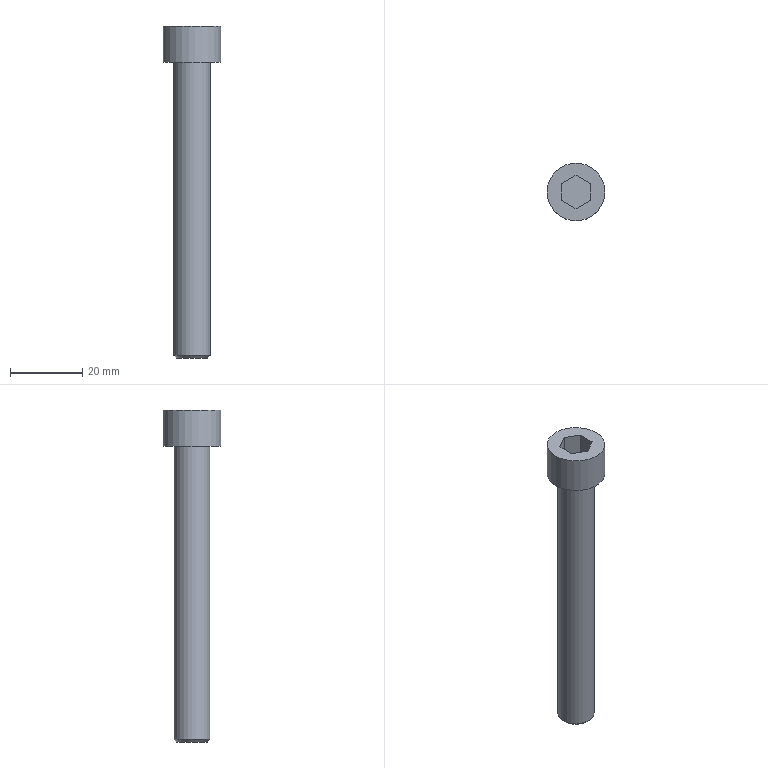Part | STEP file | gslz 2016.10.28-6_id690_x_t | 1 solid | 13 faces | box 16 x 16 x 92 mm | volume 8110 mm3 | plane 10 | cylinder 2 | cone 1 | commonest cylinder face diameters 10 x1 16 x1
STEP:
#1=CARTESIAN_POINT('',(179.7,197.309,72.));
#2=VERTEX_POINT('',#1);
#3=CARTESIAN_POINT('',(179.7,192.691,72.));
#4=VERTEX_POINT('',#3);
#5=CARTESIAN_POINT('',(179.7,197.309,72.));
#6=DIRECTION('',(0.,-1.,0.));
#7=VECTOR('',#6,1.);
#8=LINE('',#5,#7);
#9=EDGE_CURVE('',#2,#4,#8,.T.);
#10=ORIENTED_EDGE('',*,*,#9,.T.);
#11=CARTESIAN_POINT('',(175.7,190.381,72.));
#12=VERTEX_POINT('',#11);
#13=CARTESIAN_POINT('',(179.7,192.691,72.));
#14=DIRECTION('',(-0.866,-0.5,0.));
#15=VECTOR('',#14,1.);
#16=LINE('',#13,#15);
#17=EDGE_CURVE('',#4,#12,#16,.T.);
#18=ORIENTED_EDGE('',*,*,#17,.T.);
#19=CARTESIAN_POINT('',(171.7,192.691,72.));
#20=VERTEX_POINT('',#19);
#21=CARTESIAN_POINT('',(175.7,190.381,72.));
#22=DIRECTION('',(-0.866,0.5,0.));
#23=VECTOR('',#22,1.);
#24=LINE('',#21,#23);
#25=EDGE_CURVE('',#12,#20,#24,.T.);
#26=ORIENTED_EDGE('',*,*,#25,.T.);
#27=CARTESIAN_POINT('',(171.7,197.309,72.));
#28=VERTEX_POINT('',#27);
#29=CARTESIAN_POINT('',(171.7,192.691,72.));
#30=DIRECTION('',(0.,1.,0.));
#31=VECTOR('',#30,1.);
#32=LINE('',#29,#31);
#33=EDGE_CURVE('',#20,#28,#32,.T.);
#34=ORIENTED_EDGE('',*,*,#33,.T.);
#35=CARTESIAN_POINT('',(175.7,199.619,72.));
#36=VERTEX_POINT('',#35);
#37=CARTESIAN_POINT('',(171.7,197.309,72.));
#38=DIRECTION('',(0.866,0.5,0.));
#39=VECTOR('',#38,1.);
#40=LINE('',#37,#39);
#41=EDGE_CURVE('',#28,#36,#40,.T.);
#42=ORIENTED_EDGE('',*,*,#41,.T.);
#43=CARTESIAN_POINT('',(175.7,199.619,72.));
#44=DIRECTION('',(0.866,-0.5,0.));
#45=VECTOR('',#44,1.);
#46=LINE('',#43,#45);
#47=EDGE_CURVE('',#36,#2,#46,.T.);
#48=ORIENTED_EDGE('',*,*,#47,.T.);
#49=EDGE_LOOP('',(#10,#18,#26,#34,#42,#48));
#50=FACE_BOUND('',#49,.T.);
#51=CARTESIAN_POINT('',(167.7,195.,72.));
#52=VERTEX_POINT('',#51);
#53=CARTESIAN_POINT('',(175.7,195.,72.));
#54=DIRECTION('',(0.,0.,1.));
#55=DIRECTION('',(-1.,0.,0.));
#56=AXIS2_PLACEMENT_3D('',#53,#54,#55);
#57=CIRCLE('',#56,8.);
#58=EDGE_CURVE('',#52,#52,#57,.T.);
#59=ORIENTED_EDGE('',*,*,#58,.T.);
#60=EDGE_LOOP('',(#59));
#61=FACE_BOUND('',#60,.T.);
#62=CARTESIAN_POINT('',(175.7,195.,72.));
#63=DIRECTION('',(0.,0.,1.));
#64=DIRECTION('',(1.,0.,0.));
#65=AXIS2_PLACEMENT_3D('',#62,#63,#64);
#66=PLANE('',#65);
#67=ADVANCED_FACE('',(#50,#61),#66,.T.);
#68=CARTESIAN_POINT('',(179.95,195.,-20.));
#69=VERTEX_POINT('',#68);
#70=CARTESIAN_POINT('',(175.7,195.,-20.));
#71=DIRECTION('',(0.,0.,1.));
#72=DIRECTION('',(1.,0.,0.));
#73=AXIS2_PLACEMENT_3D('',#70,#71,#72);
#74=CIRCLE('',#73,4.25);
#75=EDGE_CURVE('',#69,#69,#74,.T.);
#76=ORIENTED_EDGE('',*,*,#75,.F.);
#77=EDGE_LOOP('',(#76));
#78=FACE_OUTER_BOUND('',#77,.T.);
#79=CARTESIAN_POINT('',(175.7,195.,-20.));
#80=DIRECTION('',(0.,0.,-1.));
#81=DIRECTION('',(-1.,0.,0.));
#82=AXIS2_PLACEMENT_3D('',#79,#80,#81);
#83=PLANE('',#82);
#84=ADVANCED_FACE('',(#78),#83,.T.);
#85=CARTESIAN_POINT('',(180.7,195.,-19.25));
#86=VERTEX_POINT('',#85);
#87=CARTESIAN_POINT('',(175.7,195.,-19.25));
#88=DIRECTION('',(0.,0.,-1.));
#89=DIRECTION('',(1.,0.,0.));
#90=AXIS2_PLACEMENT_3D('',#87,#88,#89);
#91=CIRCLE('',#90,5.);
#92=EDGE_CURVE('',#86,#86,#91,.T.);
#93=ORIENTED_EDGE('',*,*,#92,.F.);
#94=EDGE_LOOP('',(#93));
#95=FACE_BOUND('',#94,.T.);
#96=CARTESIAN_POINT('',(180.7,195.,62.));
#97=VERTEX_POINT('',#96);
#98=CARTESIAN_POINT('',(175.7,195.,62.));
#99=DIRECTION('',(0.,0.,1.));
#100=DIRECTION('',(1.,0.,0.));
#101=AXIS2_PLACEMENT_3D('',#98,#99,#100);
#102=CIRCLE('',#101,5.);
#103=EDGE_CURVE('',#97,#97,#102,.T.);
#104=ORIENTED_EDGE('',*,*,#103,.F.);
#105=EDGE_LOOP('',(#104));
#106=FACE_BOUND('',#105,.T.);
#107=CARTESIAN_POINT('',(175.7,195.,0.));
#108=DIRECTION('',(0.,0.,-1.));
#109=DIRECTION('',(-1.,0.,0.));
#110=AXIS2_PLACEMENT_3D('',#107,#108,#109);
#111=CYLINDRICAL_SURFACE('',#110,5.);
#112=ADVANCED_FACE('',(#95,#106),#111,.T.);
#113=ORIENTED_EDGE('',*,*,#103,.T.);
#114=EDGE_LOOP('',(#113));
#115=FACE_BOUND('',#114,.T.);
#116=CARTESIAN_POINT('',(183.7,195.,62.));
#117=VERTEX_POINT('',#116);
#118=CARTESIAN_POINT('',(175.7,195.,62.));
#119=DIRECTION('',(0.,0.,1.));
#120=DIRECTION('',(1.,0.,0.));
#121=AXIS2_PLACEMENT_3D('',#118,#119,#120);
#122=CIRCLE('',#121,8.);
#123=EDGE_CURVE('',#117,#117,#122,.T.);
#124=ORIENTED_EDGE('',*,*,#123,.F.);
#125=EDGE_LOOP('',(#124));
#126=FACE_BOUND('',#125,.T.);
#127=CARTESIAN_POINT('',(175.7,195.,62.));
#128=DIRECTION('',(0.,0.,-1.));
#129=DIRECTION('',(-1.,0.,0.));
#130=AXIS2_PLACEMENT_3D('',#127,#128,#129);
#131=PLANE('',#130);
#132=ADVANCED_FACE('',(#115,#126),#131,.T.);
#133=ORIENTED_EDGE('',*,*,#123,.T.);
#134=EDGE_LOOP('',(#133));
#135=FACE_BOUND('',#134,.T.);
#136=ORIENTED_EDGE('',*,*,#58,.F.);
#137=EDGE_LOOP('',(#136));
#138=FACE_BOUND('',#137,.T.);
#139=CARTESIAN_POINT('',(175.7,195.,75.));
#140=DIRECTION('',(0.,0.,-1.));
#141=DIRECTION('',(-1.,0.,0.));
#142=AXIS2_PLACEMENT_3D('',#139,#140,#141);
#143=CYLINDRICAL_SURFACE('',#142,8.);
#144=ADVANCED_FACE('',(#135,#138),#143,.T.);
#145=ORIENTED_EDGE('',*,*,#9,.F.);
#146=CARTESIAN_POINT('',(179.7,197.309,66.));
#147=VERTEX_POINT('',#146);
#148=CARTESIAN_POINT('',(179.7,197.309,66.));
#149=DIRECTION('',(0.,0.,-1.));
#150=VECTOR('',#149,1.);
#151=LINE('',#148,#150);
#152=EDGE_CURVE('',#2,#147,#151,.T.);
#153=ORIENTED_EDGE('',*,*,#152,.T.);
#154=CARTESIAN_POINT('',(179.7,192.691,66.));
#155=VERTEX_POINT('',#154);
#156=CARTESIAN_POINT('',(179.7,197.309,66.));
#157=DIRECTION('',(0.,1.,0.));
#158=VECTOR('',#157,1.);
#159=LINE('',#156,#158);
#160=EDGE_CURVE('',#155,#147,#159,.T.);
#161=ORIENTED_EDGE('',*,*,#160,.F.);
#162=CARTESIAN_POINT('',(179.7,192.691,66.));
#163=DIRECTION('',(0.,0.,-1.));
#164=VECTOR('',#163,1.);
#165=LINE('',#162,#164);
#166=EDGE_CURVE('',#4,#155,#165,.T.);
#167=ORIENTED_EDGE('',*,*,#166,.F.);
#168=EDGE_LOOP('',(#145,#153,#161,#167));
#169=FACE_OUTER_BOUND('',#168,.T.);
#170=CARTESIAN_POINT('',(179.7,197.309,66.));
#171=DIRECTION('',(1.,0.,0.));
#172=DIRECTION('',(0.,1.,0.));
#173=AXIS2_PLACEMENT_3D('',#170,#171,#172);
#174=PLANE('',#173);
#175=ADVANCED_FACE('',(#169),#174,.F.);
#176=ORIENTED_EDGE('',*,*,#17,.F.);
#177=ORIENTED_EDGE('',*,*,#166,.T.);
#178=CARTESIAN_POINT('',(175.7,190.381,66.));
#179=VERTEX_POINT('',#178);
#180=CARTESIAN_POINT('',(179.7,192.691,66.));
#181=DIRECTION('',(0.866,0.5,0.));
#182=VECTOR('',#181,1.);
#183=LINE('',#180,#182);
#184=EDGE_CURVE('',#179,#155,#183,.T.);
#185=ORIENTED_EDGE('',*,*,#184,.F.);
#186=CARTESIAN_POINT('',(175.7,190.381,66.));
#187=DIRECTION('',(0.,0.,-1.));
#188=VECTOR('',#187,1.);
#189=LINE('',#186,#188);
#190=EDGE_CURVE('',#12,#179,#189,.T.);
#191=ORIENTED_EDGE('',*,*,#190,.F.);
#192=EDGE_LOOP('',(#176,#177,#185,#191));
#193=FACE_OUTER_BOUND('',#192,.T.);
#194=CARTESIAN_POINT('',(179.7,192.691,66.));
#195=DIRECTION('',(0.5,-0.866,0.));
#196=DIRECTION('',(0.866,0.5,0.));
#197=AXIS2_PLACEMENT_3D('',#194,#195,#196);
#198=PLANE('',#197);
#199=ADVANCED_FACE('',(#193),#198,.F.);
#200=ORIENTED_EDGE('',*,*,#25,.F.);
#201=ORIENTED_EDGE('',*,*,#190,.T.);
#202=CARTESIAN_POINT('',(171.7,192.691,66.));
#203=VERTEX_POINT('',#202);
#204=CARTESIAN_POINT('',(175.7,190.381,66.));
#205=DIRECTION('',(0.866,-0.5,0.));
#206=VECTOR('',#205,1.);
#207=LINE('',#204,#206);
#208=EDGE_CURVE('',#203,#179,#207,.T.);
#209=ORIENTED_EDGE('',*,*,#208,.F.);
#210=CARTESIAN_POINT('',(171.7,192.691,66.));
#211=DIRECTION('',(0.,0.,-1.));
#212=VECTOR('',#211,1.);
#213=LINE('',#210,#212);
#214=EDGE_CURVE('',#20,#203,#213,.T.);
#215=ORIENTED_EDGE('',*,*,#214,.F.);
#216=EDGE_LOOP('',(#200,#201,#209,#215));
#217=FACE_OUTER_BOUND('',#216,.T.);
#218=CARTESIAN_POINT('',(175.7,190.381,66.));
#219=DIRECTION('',(-0.5,-0.866,0.));
#220=DIRECTION('',(0.866,-0.5,0.));
#221=AXIS2_PLACEMENT_3D('',#218,#219,#220);
#222=PLANE('',#221);
#223=ADVANCED_FACE('',(#217),#222,.F.);
#224=ORIENTED_EDGE('',*,*,#33,.F.);
#225=ORIENTED_EDGE('',*,*,#214,.T.);
#226=CARTESIAN_POINT('',(171.7,197.309,66.));
#227=VERTEX_POINT('',#226);
#228=CARTESIAN_POINT('',(171.7,192.691,66.));
#229=DIRECTION('',(0.,-1.,0.));
#230=VECTOR('',#229,1.);
#231=LINE('',#228,#230);
#232=EDGE_CURVE('',#227,#203,#231,.T.);
#233=ORIENTED_EDGE('',*,*,#232,.F.);
#234=CARTESIAN_POINT('',(171.7,197.309,66.));
#235=DIRECTION('',(0.,0.,-1.));
#236=VECTOR('',#235,1.);
#237=LINE('',#234,#236);
#238=EDGE_CURVE('',#28,#227,#237,.T.);
#239=ORIENTED_EDGE('',*,*,#238,.F.);
#240=EDGE_LOOP('',(#224,#225,#233,#239));
#241=FACE_OUTER_BOUND('',#240,.T.);
#242=CARTESIAN_POINT('',(171.7,192.691,66.));
#243=DIRECTION('',(-1.,0.,0.));
#244=DIRECTION('',(0.,0.,1.));
#245=AXIS2_PLACEMENT_3D('',#242,#243,#244);
#246=PLANE('',#245);
#247=ADVANCED_FACE('',(#241),#246,.F.);
#248=ORIENTED_EDGE('',*,*,#41,.F.);
#249=ORIENTED_EDGE('',*,*,#238,.T.);
#250=CARTESIAN_POINT('',(175.7,199.619,66.));
#251=VERTEX_POINT('',#250);
#252=CARTESIAN_POINT('',(171.7,197.309,66.));
#253=DIRECTION('',(-0.866,-0.5,0.));
#254=VECTOR('',#253,1.);
#255=LINE('',#252,#254);
#256=EDGE_CURVE('',#251,#227,#255,.T.);
#257=ORIENTED_EDGE('',*,*,#256,.F.);
#258=CARTESIAN_POINT('',(175.7,199.619,66.));
#259=DIRECTION('',(0.,0.,-1.));
#260=VECTOR('',#259,1.);
#261=LINE('',#258,#260);
#262=EDGE_CURVE('',#36,#251,#261,.T.);
#263=ORIENTED_EDGE('',*,*,#262,.F.);
#264=EDGE_LOOP('',(#248,#249,#257,#263));
#265=FACE_OUTER_BOUND('',#264,.T.);
#266=CARTESIAN_POINT('',(171.7,197.309,66.));
#267=DIRECTION('',(-0.5,0.866,0.));
#268=DIRECTION('',(-0.866,-0.5,0.));
#269=AXIS2_PLACEMENT_3D('',#266,#267,#268);
#270=PLANE('',#269);
#271=ADVANCED_FACE('',(#265),#270,.F.);
#272=ORIENTED_EDGE('',*,*,#47,.F.);
#273=ORIENTED_EDGE('',*,*,#262,.T.);
#274=CARTESIAN_POINT('',(175.7,199.619,66.));
#275=DIRECTION('',(-0.866,0.5,0.));
#276=VECTOR('',#275,1.);
#277=LINE('',#274,#276);
#278=EDGE_CURVE('',#147,#251,#277,.T.);
#279=ORIENTED_EDGE('',*,*,#278,.F.);
#280=ORIENTED_EDGE('',*,*,#152,.F.);
#281=EDGE_LOOP('',(#272,#273,#279,#280));
#282=FACE_OUTER_BOUND('',#281,.T.);
#283=CARTESIAN_POINT('',(175.7,199.619,66.));
#284=DIRECTION('',(0.5,0.866,0.));
#285=DIRECTION('',(-0.866,0.5,0.));
#286=AXIS2_PLACEMENT_3D('',#283,#284,#285);
#287=PLANE('',#286);
#288=ADVANCED_FACE('',(#282),#287,.F.);
#289=ORIENTED_EDGE('',*,*,#160,.T.);
#290=ORIENTED_EDGE('',*,*,#278,.T.);
#291=ORIENTED_EDGE('',*,*,#256,.T.);
#292=ORIENTED_EDGE('',*,*,#232,.T.);
#293=ORIENTED_EDGE('',*,*,#208,.T.);
#294=ORIENTED_EDGE('',*,*,#184,.T.);
#295=EDGE_LOOP('',(#289,#290,#291,#292,#293,#294));
#296=FACE_OUTER_BOUND('',#295,.T.);
#297=CARTESIAN_POINT('',(179.7,192.691,66.));
#298=DIRECTION('',(0.,0.,1.));
#299=DIRECTION('',(1.,0.,0.));
#300=AXIS2_PLACEMENT_3D('',#297,#298,#299);
#301=PLANE('',#300);
#302=ADVANCED_FACE('',(#296),#301,.T.);
#303=ORIENTED_EDGE('',*,*,#92,.T.);
#304=EDGE_LOOP('',(#303));
#305=FACE_BOUND('',#304,.T.);
#306=ORIENTED_EDGE('',*,*,#75,.T.);
#307=EDGE_LOOP('',(#306));
#308=FACE_BOUND('',#307,.T.);
#309=CARTESIAN_POINT('',(175.7,195.,-20.));
#310=DIRECTION('',(0.,0.,1.));
#311=DIRECTION('',(1.,0.,0.));
#312=AXIS2_PLACEMENT_3D('',#309,#310,#311);
#313=CONICAL_SURFACE('',#312,4.25,45.);
#314=ADVANCED_FACE('',(#305,#308),#313,.T.);
#315=CLOSED_SHELL('',(#67,#84,#112,#132,#144,#175,#199,#223,#247,#271,#288,#302,#314));
#316=MANIFOLD_SOLID_BREP('',#315);
#317=(LENGTH_UNIT()NAMED_UNIT(*)SI_UNIT(.MILLI.,.METRE.));
#318=UNCERTAINTY_MEASURE_WITH_UNIT(LENGTH_MEASURE(0.00002),#317,'','');
#319=(NAMED_UNIT(*)PLANE_ANGLE_UNIT()SI_UNIT($,.RADIAN.));
#320=PLANE_ANGLE_MEASURE_WITH_UNIT(PLANE_ANGLE_MEASURE(0.01745),#319);
#321=DIMENSIONAL_EXPONENTS(0.,0.,0.,0.,0.,0.,0.);
#322=(CONVERSION_BASED_UNIT('DEGREE',#320)NAMED_UNIT(#321)PLANE_ANGLE_UNIT());
#323=(NAMED_UNIT(*)SI_UNIT($,.STERADIAN.)SOLID_ANGLE_UNIT());
#324=(GEOMETRIC_REPRESENTATION_CONTEXT(3)GLOBAL_UNCERTAINTY_ASSIGNED_CONTEXT((#318))GLOBAL_UNIT_ASSIGNED_CONTEXT((#317,#322,#323))REPRESENTATION_CONTEXT('',''));
#325=ADVANCED_BREP_SHAPE_REPRESENTATION('',(#316),#324);